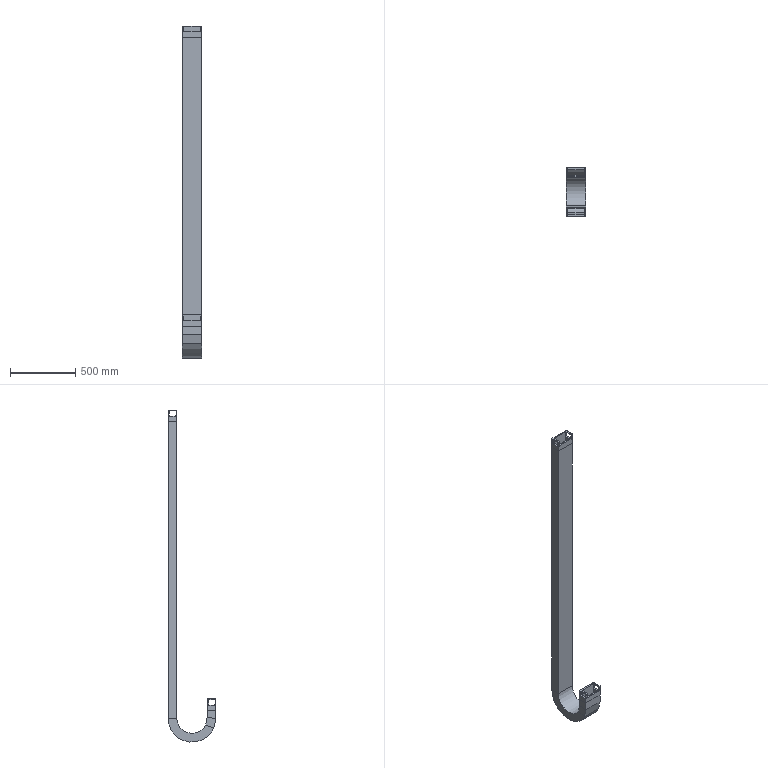Part | STEP file | 45C.125.150-42-45C.125.12PZ | 3 solids | 132 faces | box 153 x 367 x 2542 mm | volume 13515724 mm3 | plane 80 | cylinder 50 | spline 2 | commonest cylinder face diameters 6.5 x48 233 x1 255 x1